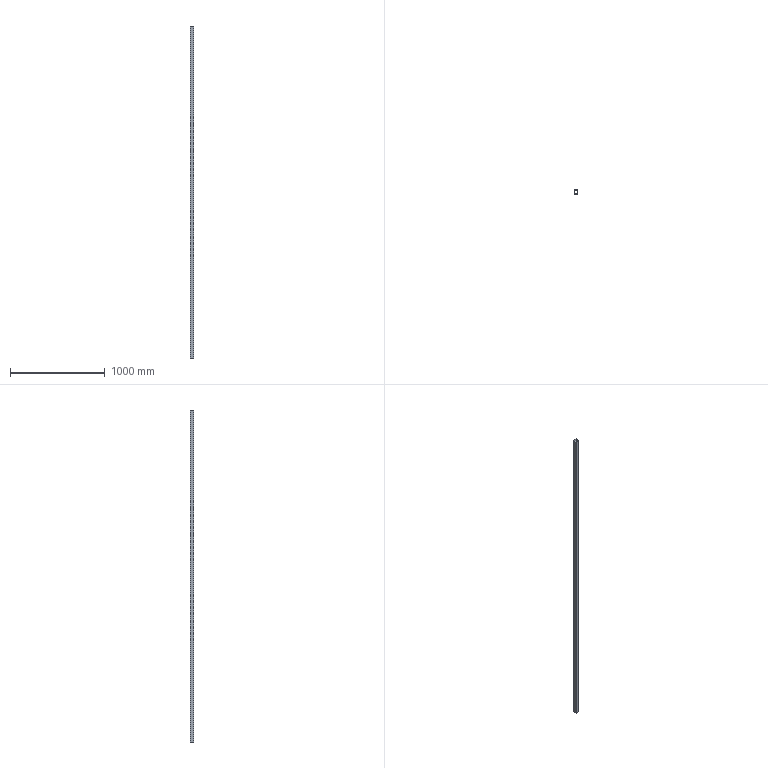Part | STEP file | BCC3 H18_1 | 1 solid | 10 faces | box 40 x 40 x 3500 mm | volume 1554000 mm3 | plane 10
STEP:
#1=CARTESIAN_POINT('',(0.,0.,0.));
#2=DIRECTION('',(0.,0.,1.));
#3=DIRECTION('',(1.,0.,0.));
#4=AXIS2_PLACEMENT_3D('',#1,#2,#3);
#5=CARTESIAN_POINT('',(-20.,20.,1750.));
#6=VERTEX_POINT('',#5);
#7=CARTESIAN_POINT('',(-20.,-20.,1750.));
#8=VERTEX_POINT('',#7);
#9=CARTESIAN_POINT('',(-20.,20.,1750.));
#10=DIRECTION('',(0.,-1.,0.));
#11=VECTOR('',#10,1.);
#12=LINE('',#9,#11);
#13=CARTESIAN_POINT('',(0.,0.,1750.));
#14=DIRECTION('',(0.,0.,1.));
#15=DIRECTION('',(1.,0.,0.));
#16=AXIS2_PLACEMENT_3D('',#13,#14,#15);
#17=PLANE('',#16);
#18=CARTESIAN_POINT('',(-20.,20.));
#19=DIRECTION('',(0.,-1.));
#20=VECTOR('',#19,1.);
#21=LINE('',#18,#20);
#22=(GEOMETRIC_REPRESENTATION_CONTEXT(2)PARAMETRIC_REPRESENTATION_CONTEXT()REPRESENTATION_CONTEXT('',''));
#23=DEFINITIONAL_REPRESENTATION('',(#21),#22);
#24=PCURVE('',#17,#23);
#25=CARTESIAN_POINT('',(-20.,20.,1750.));
#26=DIRECTION('',(1.,0.,0.));
#27=DIRECTION('',(0.,1.,0.));
#28=AXIS2_PLACEMENT_3D('',#25,#26,#27);
#29=PLANE('',#28);
#30=CARTESIAN_POINT('',(0.,0.));
#31=DIRECTION('',(-1.,0.));
#32=VECTOR('',#31,1.);
#33=LINE('',#30,#32);
#34=(GEOMETRIC_REPRESENTATION_CONTEXT(2)PARAMETRIC_REPRESENTATION_CONTEXT()REPRESENTATION_CONTEXT('',''));
#35=DEFINITIONAL_REPRESENTATION('',(#33),#34);
#36=PCURVE('',#29,#35);
#37=SURFACE_CURVE('',#12,(#24,#36),.PCURVE_S1.);
#38=EDGE_CURVE('',#6,#8,#37,.T.);
#39=ORIENTED_EDGE('',*,*,#38,.T.);
#40=CARTESIAN_POINT('',(20.,-20.,1750.));
#41=VERTEX_POINT('',#40);
#42=CARTESIAN_POINT('',(-20.,-20.,1750.));
#43=DIRECTION('',(1.,0.,0.));
#44=VECTOR('',#43,1.);
#45=LINE('',#42,#44);
#46=CARTESIAN_POINT('',(-20.,-20.));
#47=DIRECTION('',(1.,0.));
#48=VECTOR('',#47,1.);
#49=LINE('',#46,#48);
#50=(GEOMETRIC_REPRESENTATION_CONTEXT(2)PARAMETRIC_REPRESENTATION_CONTEXT()REPRESENTATION_CONTEXT('',''));
#51=DEFINITIONAL_REPRESENTATION('',(#49),#50);
#52=PCURVE('',#17,#51);
#53=CARTESIAN_POINT('',(-20.,-20.,1750.));
#54=DIRECTION('',(0.,1.,0.));
#55=DIRECTION('',(0.,0.,1.));
#56=AXIS2_PLACEMENT_3D('',#53,#54,#55);
#57=PLANE('',#56);
#58=CARTESIAN_POINT('',(0.,0.));
#59=DIRECTION('',(0.,1.));
#60=VECTOR('',#59,1.);
#61=LINE('',#58,#60);
#62=(GEOMETRIC_REPRESENTATION_CONTEXT(2)PARAMETRIC_REPRESENTATION_CONTEXT()REPRESENTATION_CONTEXT('',''));
#63=DEFINITIONAL_REPRESENTATION('',(#61),#62);
#64=PCURVE('',#57,#63);
#65=SURFACE_CURVE('',#45,(#52,#64),.PCURVE_S1.);
#66=EDGE_CURVE('',#8,#41,#65,.T.);
#67=ORIENTED_EDGE('',*,*,#66,.T.);
#68=CARTESIAN_POINT('',(20.,20.,1750.));
#69=VERTEX_POINT('',#68);
#70=CARTESIAN_POINT('',(20.,20.,1750.));
#71=DIRECTION('',(0.,1.,0.));
#72=VECTOR('',#71,1.);
#73=LINE('',#70,#72);
#74=CARTESIAN_POINT('',(20.,20.));
#75=DIRECTION('',(0.,1.));
#76=VECTOR('',#75,1.);
#77=LINE('',#74,#76);
#78=(GEOMETRIC_REPRESENTATION_CONTEXT(2)PARAMETRIC_REPRESENTATION_CONTEXT()REPRESENTATION_CONTEXT('',''));
#79=DEFINITIONAL_REPRESENTATION('',(#77),#78);
#80=PCURVE('',#17,#79);
#81=CARTESIAN_POINT('',(20.,20.,1750.));
#82=DIRECTION('',(-1.,0.,0.));
#83=DIRECTION('',(0.,-1.,0.));
#84=AXIS2_PLACEMENT_3D('',#81,#82,#83);
#85=PLANE('',#84);
#86=CARTESIAN_POINT('',(0.,0.));
#87=DIRECTION('',(-1.,0.));
#88=VECTOR('',#87,1.);
#89=LINE('',#86,#88);
#90=(GEOMETRIC_REPRESENTATION_CONTEXT(2)PARAMETRIC_REPRESENTATION_CONTEXT()REPRESENTATION_CONTEXT('',''));
#91=DEFINITIONAL_REPRESENTATION('',(#89),#90);
#92=PCURVE('',#85,#91);
#93=SURFACE_CURVE('',#73,(#80,#92),.PCURVE_S1.);
#94=EDGE_CURVE('',#41,#69,#93,.T.);
#95=ORIENTED_EDGE('',*,*,#94,.T.);
#96=CARTESIAN_POINT('',(-20.,20.,1750.));
#97=DIRECTION('',(-1.,0.,0.));
#98=VECTOR('',#97,1.);
#99=LINE('',#96,#98);
#100=CARTESIAN_POINT('',(-20.,20.));
#101=DIRECTION('',(-1.,0.));
#102=VECTOR('',#101,1.);
#103=LINE('',#100,#102);
#104=(GEOMETRIC_REPRESENTATION_CONTEXT(2)PARAMETRIC_REPRESENTATION_CONTEXT()REPRESENTATION_CONTEXT('',''));
#105=DEFINITIONAL_REPRESENTATION('',(#103),#104);
#106=PCURVE('',#17,#105);
#107=CARTESIAN_POINT('',(-20.,20.,1750.));
#108=DIRECTION('',(0.,-1.,0.));
#109=DIRECTION('',(0.,0.,-1.));
#110=AXIS2_PLACEMENT_3D('',#107,#108,#109);
#111=PLANE('',#110);
#112=CARTESIAN_POINT('',(0.,0.));
#113=DIRECTION('',(0.,-1.));
#114=VECTOR('',#113,1.);
#115=LINE('',#112,#114);
#116=(GEOMETRIC_REPRESENTATION_CONTEXT(2)PARAMETRIC_REPRESENTATION_CONTEXT()REPRESENTATION_CONTEXT('',''));
#117=DEFINITIONAL_REPRESENTATION('',(#115),#116);
#118=PCURVE('',#111,#117);
#119=SURFACE_CURVE('',#99,(#106,#118),.PCURVE_S1.);
#120=EDGE_CURVE('',#69,#6,#119,.T.);
#121=ORIENTED_EDGE('',*,*,#120,.T.);
#122=EDGE_LOOP('',(#39,#67,#95,#121));
#123=FACE_BOUND('',#122,.T.);
#124=CARTESIAN_POINT('',(-17.,-17.,1750.));
#125=VERTEX_POINT('',#124);
#126=CARTESIAN_POINT('',(17.,-17.,1750.));
#127=VERTEX_POINT('',#126);
#128=CARTESIAN_POINT('',(-17.,-17.,1750.));
#129=DIRECTION('',(1.,0.,0.));
#130=VECTOR('',#129,1.);
#131=LINE('',#128,#130);
#132=CARTESIAN_POINT('',(-17.,-17.));
#133=DIRECTION('',(1.,0.));
#134=VECTOR('',#133,1.);
#135=LINE('',#132,#134);
#136=(GEOMETRIC_REPRESENTATION_CONTEXT(2)PARAMETRIC_REPRESENTATION_CONTEXT()REPRESENTATION_CONTEXT('',''));
#137=DEFINITIONAL_REPRESENTATION('',(#135),#136);
#138=PCURVE('',#17,#137);
#139=CARTESIAN_POINT('',(-17.,-17.,1750.));
#140=DIRECTION('',(0.,1.,0.));
#141=DIRECTION('',(-1.,0.,0.));
#142=AXIS2_PLACEMENT_3D('',#139,#140,#141);
#143=PLANE('',#142);
#144=CARTESIAN_POINT('',(0.,0.));
#145=DIRECTION('',(-1.,0.));
#146=VECTOR('',#145,1.);
#147=LINE('',#144,#146);
#148=(GEOMETRIC_REPRESENTATION_CONTEXT(2)PARAMETRIC_REPRESENTATION_CONTEXT()REPRESENTATION_CONTEXT('',''));
#149=DEFINITIONAL_REPRESENTATION('',(#147),#148);
#150=PCURVE('',#143,#149);
#151=SURFACE_CURVE('',#131,(#138,#150),.PCURVE_S1.);
#152=EDGE_CURVE('',#125,#127,#151,.T.);
#153=ORIENTED_EDGE('',*,*,#152,.F.);
#154=CARTESIAN_POINT('',(-17.,17.,1750.));
#155=VERTEX_POINT('',#154);
#156=CARTESIAN_POINT('',(-17.,17.,1750.));
#157=DIRECTION('',(0.,-1.,0.));
#158=VECTOR('',#157,1.);
#159=LINE('',#156,#158);
#160=CARTESIAN_POINT('',(-17.,17.));
#161=DIRECTION('',(0.,-1.));
#162=VECTOR('',#161,1.);
#163=LINE('',#160,#162);
#164=(GEOMETRIC_REPRESENTATION_CONTEXT(2)PARAMETRIC_REPRESENTATION_CONTEXT()REPRESENTATION_CONTEXT('',''));
#165=DEFINITIONAL_REPRESENTATION('',(#163),#164);
#166=PCURVE('',#17,#165);
#167=CARTESIAN_POINT('',(-17.,17.,1750.));
#168=DIRECTION('',(1.,0.,0.));
#169=DIRECTION('',(0.,1.,0.));
#170=AXIS2_PLACEMENT_3D('',#167,#168,#169);
#171=PLANE('',#170);
#172=CARTESIAN_POINT('',(0.,0.));
#173=DIRECTION('',(-1.,0.));
#174=VECTOR('',#173,1.);
#175=LINE('',#172,#174);
#176=(GEOMETRIC_REPRESENTATION_CONTEXT(2)PARAMETRIC_REPRESENTATION_CONTEXT()REPRESENTATION_CONTEXT('',''));
#177=DEFINITIONAL_REPRESENTATION('',(#175),#176);
#178=PCURVE('',#171,#177);
#179=SURFACE_CURVE('',#159,(#166,#178),.PCURVE_S1.);
#180=EDGE_CURVE('',#155,#125,#179,.T.);
#181=ORIENTED_EDGE('',*,*,#180,.F.);
#182=CARTESIAN_POINT('',(17.,17.,1750.));
#183=VERTEX_POINT('',#182);
#184=CARTESIAN_POINT('',(-17.,17.,1750.));
#185=DIRECTION('',(-1.,0.,0.));
#186=VECTOR('',#185,1.);
#187=LINE('',#184,#186);
#188=CARTESIAN_POINT('',(-17.,17.));
#189=DIRECTION('',(-1.,0.));
#190=VECTOR('',#189,1.);
#191=LINE('',#188,#190);
#192=(GEOMETRIC_REPRESENTATION_CONTEXT(2)PARAMETRIC_REPRESENTATION_CONTEXT()REPRESENTATION_CONTEXT('',''));
#193=DEFINITIONAL_REPRESENTATION('',(#191),#192);
#194=PCURVE('',#17,#193);
#195=CARTESIAN_POINT('',(-17.,17.,1750.));
#196=DIRECTION('',(0.,-1.,0.));
#197=DIRECTION('',(0.,0.,-1.));
#198=AXIS2_PLACEMENT_3D('',#195,#196,#197);
#199=PLANE('',#198);
#200=CARTESIAN_POINT('',(0.,0.));
#201=DIRECTION('',(0.,-1.));
#202=VECTOR('',#201,1.);
#203=LINE('',#200,#202);
#204=(GEOMETRIC_REPRESENTATION_CONTEXT(2)PARAMETRIC_REPRESENTATION_CONTEXT()REPRESENTATION_CONTEXT('',''));
#205=DEFINITIONAL_REPRESENTATION('',(#203),#204);
#206=PCURVE('',#199,#205);
#207=SURFACE_CURVE('',#187,(#194,#206),.PCURVE_S1.);
#208=EDGE_CURVE('',#183,#155,#207,.T.);
#209=ORIENTED_EDGE('',*,*,#208,.F.);
#210=CARTESIAN_POINT('',(17.,17.,1750.));
#211=DIRECTION('',(0.,1.,0.));
#212=VECTOR('',#211,1.);
#213=LINE('',#210,#212);
#214=CARTESIAN_POINT('',(17.,17.));
#215=DIRECTION('',(0.,1.));
#216=VECTOR('',#215,1.);
#217=LINE('',#214,#216);
#218=(GEOMETRIC_REPRESENTATION_CONTEXT(2)PARAMETRIC_REPRESENTATION_CONTEXT()REPRESENTATION_CONTEXT('',''));
#219=DEFINITIONAL_REPRESENTATION('',(#217),#218);
#220=PCURVE('',#17,#219);
#221=CARTESIAN_POINT('',(17.,17.,1750.));
#222=DIRECTION('',(-1.,0.,0.));
#223=DIRECTION('',(0.,-1.,0.));
#224=AXIS2_PLACEMENT_3D('',#221,#222,#223);
#225=PLANE('',#224);
#226=CARTESIAN_POINT('',(0.,0.));
#227=DIRECTION('',(-1.,0.));
#228=VECTOR('',#227,1.);
#229=LINE('',#226,#228);
#230=(GEOMETRIC_REPRESENTATION_CONTEXT(2)PARAMETRIC_REPRESENTATION_CONTEXT()REPRESENTATION_CONTEXT('',''));
#231=DEFINITIONAL_REPRESENTATION('',(#229),#230);
#232=PCURVE('',#225,#231);
#233=SURFACE_CURVE('',#213,(#220,#232),.PCURVE_S1.);
#234=EDGE_CURVE('',#127,#183,#233,.T.);
#235=ORIENTED_EDGE('',*,*,#234,.F.);
#236=EDGE_LOOP('',(#153,#181,#209,#235));
#237=FACE_BOUND('',#236,.T.);
#238=ADVANCED_FACE('',(#123,#237),#17,.T.);
#239=CARTESIAN_POINT('',(-20.,20.,-1750.));
#240=VERTEX_POINT('',#239);
#241=CARTESIAN_POINT('',(-20.,-20.,-1750.));
#242=VERTEX_POINT('',#241);
#243=CARTESIAN_POINT('',(-20.,20.,-1750.));
#244=DIRECTION('',(0.,-1.,0.));
#245=VECTOR('',#244,1.);
#246=LINE('',#243,#245);
#247=CARTESIAN_POINT('',(0.,0.,-1750.));
#248=DIRECTION('',(0.,0.,1.));
#249=DIRECTION('',(1.,0.,0.));
#250=AXIS2_PLACEMENT_3D('',#247,#248,#249);
#251=PLANE('',#250);
#252=CARTESIAN_POINT('',(-20.,20.));
#253=DIRECTION('',(0.,-1.));
#254=VECTOR('',#253,1.);
#255=LINE('',#252,#254);
#256=(GEOMETRIC_REPRESENTATION_CONTEXT(2)PARAMETRIC_REPRESENTATION_CONTEXT()REPRESENTATION_CONTEXT('',''));
#257=DEFINITIONAL_REPRESENTATION('',(#255),#256);
#258=PCURVE('',#251,#257);
#259=CARTESIAN_POINT('',(0.,-3500.));
#260=DIRECTION('',(-1.,0.));
#261=VECTOR('',#260,1.);
#262=LINE('',#259,#261);
#263=(GEOMETRIC_REPRESENTATION_CONTEXT(2)PARAMETRIC_REPRESENTATION_CONTEXT()REPRESENTATION_CONTEXT('',''));
#264=DEFINITIONAL_REPRESENTATION('',(#262),#263);
#265=PCURVE('',#29,#264);
#266=SURFACE_CURVE('',#246,(#258,#265),.PCURVE_S1.);
#267=EDGE_CURVE('',#240,#242,#266,.T.);
#268=ORIENTED_EDGE('',*,*,#267,.F.);
#269=CARTESIAN_POINT('',(20.,20.,-1750.));
#270=VERTEX_POINT('',#269);
#271=CARTESIAN_POINT('',(-20.,20.,-1750.));
#272=DIRECTION('',(-1.,0.,0.));
#273=VECTOR('',#272,1.);
#274=LINE('',#271,#273);
#275=CARTESIAN_POINT('',(-20.,20.));
#276=DIRECTION('',(-1.,0.));
#277=VECTOR('',#276,1.);
#278=LINE('',#275,#277);
#279=(GEOMETRIC_REPRESENTATION_CONTEXT(2)PARAMETRIC_REPRESENTATION_CONTEXT()REPRESENTATION_CONTEXT('',''));
#280=DEFINITIONAL_REPRESENTATION('',(#278),#279);
#281=PCURVE('',#251,#280);
#282=CARTESIAN_POINT('',(3500.,0.));
#283=DIRECTION('',(0.,-1.));
#284=VECTOR('',#283,1.);
#285=LINE('',#282,#284);
#286=(GEOMETRIC_REPRESENTATION_CONTEXT(2)PARAMETRIC_REPRESENTATION_CONTEXT()REPRESENTATION_CONTEXT('',''));
#287=DEFINITIONAL_REPRESENTATION('',(#285),#286);
#288=PCURVE('',#111,#287);
#289=SURFACE_CURVE('',#274,(#281,#288),.PCURVE_S1.);
#290=EDGE_CURVE('',#270,#240,#289,.T.);
#291=ORIENTED_EDGE('',*,*,#290,.F.);
#292=CARTESIAN_POINT('',(20.,-20.,-1750.));
#293=VERTEX_POINT('',#292);
#294=CARTESIAN_POINT('',(20.,20.,-1750.));
#295=DIRECTION('',(0.,1.,0.));
#296=VECTOR('',#295,1.);
#297=LINE('',#294,#296);
#298=CARTESIAN_POINT('',(20.,20.));
#299=DIRECTION('',(0.,1.));
#300=VECTOR('',#299,1.);
#301=LINE('',#298,#300);
#302=(GEOMETRIC_REPRESENTATION_CONTEXT(2)PARAMETRIC_REPRESENTATION_CONTEXT()REPRESENTATION_CONTEXT('',''));
#303=DEFINITIONAL_REPRESENTATION('',(#301),#302);
#304=PCURVE('',#251,#303);
#305=CARTESIAN_POINT('',(0.,-3500.));
#306=DIRECTION('',(-1.,0.));
#307=VECTOR('',#306,1.);
#308=LINE('',#305,#307);
#309=(GEOMETRIC_REPRESENTATION_CONTEXT(2)PARAMETRIC_REPRESENTATION_CONTEXT()REPRESENTATION_CONTEXT('',''));
#310=DEFINITIONAL_REPRESENTATION('',(#308),#309);
#311=PCURVE('',#85,#310);
#312=SURFACE_CURVE('',#297,(#304,#311),.PCURVE_S1.);
#313=EDGE_CURVE('',#293,#270,#312,.T.);
#314=ORIENTED_EDGE('',*,*,#313,.F.);
#315=CARTESIAN_POINT('',(-20.,-20.,-1750.));
#316=DIRECTION('',(1.,0.,0.));
#317=VECTOR('',#316,1.);
#318=LINE('',#315,#317);
#319=CARTESIAN_POINT('',(-20.,-20.));
#320=DIRECTION('',(1.,0.));
#321=VECTOR('',#320,1.);
#322=LINE('',#319,#321);
#323=(GEOMETRIC_REPRESENTATION_CONTEXT(2)PARAMETRIC_REPRESENTATION_CONTEXT()REPRESENTATION_CONTEXT('',''));
#324=DEFINITIONAL_REPRESENTATION('',(#322),#323);
#325=PCURVE('',#251,#324);
#326=CARTESIAN_POINT('',(-3500.,0.));
#327=DIRECTION('',(0.,1.));
#328=VECTOR('',#327,1.);
#329=LINE('',#326,#328);
#330=(GEOMETRIC_REPRESENTATION_CONTEXT(2)PARAMETRIC_REPRESENTATION_CONTEXT()REPRESENTATION_CONTEXT('',''));
#331=DEFINITIONAL_REPRESENTATION('',(#329),#330);
#332=PCURVE('',#57,#331);
#333=SURFACE_CURVE('',#318,(#325,#332),.PCURVE_S1.);
#334=EDGE_CURVE('',#242,#293,#333,.T.);
#335=ORIENTED_EDGE('',*,*,#334,.F.);
#336=EDGE_LOOP('',(#268,#291,#314,#335));
#337=FACE_BOUND('',#336,.T.);
#338=CARTESIAN_POINT('',(-17.,17.,-1750.));
#339=VERTEX_POINT('',#338);
#340=CARTESIAN_POINT('',(-17.,-17.,-1750.));
#341=VERTEX_POINT('',#340);
#342=CARTESIAN_POINT('',(-17.,17.,-1750.));
#343=DIRECTION('',(0.,-1.,0.));
#344=VECTOR('',#343,1.);
#345=LINE('',#342,#344);
#346=CARTESIAN_POINT('',(-17.,17.));
#347=DIRECTION('',(0.,-1.));
#348=VECTOR('',#347,1.);
#349=LINE('',#346,#348);
#350=(GEOMETRIC_REPRESENTATION_CONTEXT(2)PARAMETRIC_REPRESENTATION_CONTEXT()REPRESENTATION_CONTEXT('',''));
#351=DEFINITIONAL_REPRESENTATION('',(#349),#350);
#352=PCURVE('',#251,#351);
#353=CARTESIAN_POINT('',(0.,-3500.));
#354=DIRECTION('',(-1.,0.));
#355=VECTOR('',#354,1.);
#356=LINE('',#353,#355);
#357=(GEOMETRIC_REPRESENTATION_CONTEXT(2)PARAMETRIC_REPRESENTATION_CONTEXT()REPRESENTATION_CONTEXT('',''));
#358=DEFINITIONAL_REPRESENTATION('',(#356),#357);
#359=PCURVE('',#171,#358);
#360=SURFACE_CURVE('',#345,(#352,#359),.PCURVE_S1.);
#361=EDGE_CURVE('',#339,#341,#360,.T.);
#362=ORIENTED_EDGE('',*,*,#361,.T.);
#363=CARTESIAN_POINT('',(17.,-17.,-1750.));
#364=VERTEX_POINT('',#363);
#365=CARTESIAN_POINT('',(-17.,-17.,-1750.));
#366=DIRECTION('',(1.,0.,0.));
#367=VECTOR('',#366,1.);
#368=LINE('',#365,#367);
#369=CARTESIAN_POINT('',(-17.,-17.));
#370=DIRECTION('',(1.,0.));
#371=VECTOR('',#370,1.);
#372=LINE('',#369,#371);
#373=(GEOMETRIC_REPRESENTATION_CONTEXT(2)PARAMETRIC_REPRESENTATION_CONTEXT()REPRESENTATION_CONTEXT('',''));
#374=DEFINITIONAL_REPRESENTATION('',(#372),#373);
#375=PCURVE('',#251,#374);
#376=CARTESIAN_POINT('',(0.,-3500.));
#377=DIRECTION('',(-1.,0.));
#378=VECTOR('',#377,1.);
#379=LINE('',#376,#378);
#380=(GEOMETRIC_REPRESENTATION_CONTEXT(2)PARAMETRIC_REPRESENTATION_CONTEXT()REPRESENTATION_CONTEXT('',''));
#381=DEFINITIONAL_REPRESENTATION('',(#379),#380);
#382=PCURVE('',#143,#381);
#383=SURFACE_CURVE('',#368,(#375,#382),.PCURVE_S1.);
#384=EDGE_CURVE('',#341,#364,#383,.T.);
#385=ORIENTED_EDGE('',*,*,#384,.T.);
#386=CARTESIAN_POINT('',(17.,17.,-1750.));
#387=VERTEX_POINT('',#386);
#388=CARTESIAN_POINT('',(17.,17.,-1750.));
#389=DIRECTION('',(0.,1.,0.));
#390=VECTOR('',#389,1.);
#391=LINE('',#388,#390);
#392=CARTESIAN_POINT('',(17.,17.));
#393=DIRECTION('',(0.,1.));
#394=VECTOR('',#393,1.);
#395=LINE('',#392,#394);
#396=(GEOMETRIC_REPRESENTATION_CONTEXT(2)PARAMETRIC_REPRESENTATION_CONTEXT()REPRESENTATION_CONTEXT('',''));
#397=DEFINITIONAL_REPRESENTATION('',(#395),#396);
#398=PCURVE('',#251,#397);
#399=CARTESIAN_POINT('',(0.,-3500.));
#400=DIRECTION('',(-1.,0.));
#401=VECTOR('',#400,1.);
#402=LINE('',#399,#401);
#403=(GEOMETRIC_REPRESENTATION_CONTEXT(2)PARAMETRIC_REPRESENTATION_CONTEXT()REPRESENTATION_CONTEXT('',''));
#404=DEFINITIONAL_REPRESENTATION('',(#402),#403);
#405=PCURVE('',#225,#404);
#406=SURFACE_CURVE('',#391,(#398,#405),.PCURVE_S1.);
#407=EDGE_CURVE('',#364,#387,#406,.T.);
#408=ORIENTED_EDGE('',*,*,#407,.T.);
#409=CARTESIAN_POINT('',(-17.,17.,-1750.));
#410=DIRECTION('',(-1.,0.,0.));
#411=VECTOR('',#410,1.);
#412=LINE('',#409,#411);
#413=CARTESIAN_POINT('',(-17.,17.));
#414=DIRECTION('',(-1.,0.));
#415=VECTOR('',#414,1.);
#416=LINE('',#413,#415);
#417=(GEOMETRIC_REPRESENTATION_CONTEXT(2)PARAMETRIC_REPRESENTATION_CONTEXT()REPRESENTATION_CONTEXT('',''));
#418=DEFINITIONAL_REPRESENTATION('',(#416),#417);
#419=PCURVE('',#251,#418);
#420=CARTESIAN_POINT('',(3500.,0.));
#421=DIRECTION('',(0.,-1.));
#422=VECTOR('',#421,1.);
#423=LINE('',#420,#422);
#424=(GEOMETRIC_REPRESENTATION_CONTEXT(2)PARAMETRIC_REPRESENTATION_CONTEXT()REPRESENTATION_CONTEXT('',''));
#425=DEFINITIONAL_REPRESENTATION('',(#423),#424);
#426=PCURVE('',#199,#425);
#427=SURFACE_CURVE('',#412,(#419,#426),.PCURVE_S1.);
#428=EDGE_CURVE('',#387,#339,#427,.T.);
#429=ORIENTED_EDGE('',*,*,#428,.T.);
#430=EDGE_LOOP('',(#362,#385,#408,#429));
#431=FACE_BOUND('',#430,.T.);
#432=ADVANCED_FACE('',(#337,#431),#251,.F.);
#433=ORIENTED_EDGE('',*,*,#267,.T.);
#434=CARTESIAN_POINT('',(-20.,-20.,1750.));
#435=DIRECTION('',(0.,0.,-1.));
#436=VECTOR('',#435,1.);
#437=LINE('',#434,#436);
#438=CARTESIAN_POINT('',(-40.,0.));
#439=DIRECTION('',(0.,-1.));
#440=VECTOR('',#439,1.);
#441=LINE('',#438,#440);
#442=(GEOMETRIC_REPRESENTATION_CONTEXT(2)PARAMETRIC_REPRESENTATION_CONTEXT()REPRESENTATION_CONTEXT('',''));
#443=DEFINITIONAL_REPRESENTATION('',(#441),#442);
#444=PCURVE('',#29,#443);
#445=CARTESIAN_POINT('',(0.,0.));
#446=DIRECTION('',(-1.,0.));
#447=VECTOR('',#446,1.);
#448=LINE('',#445,#447);
#449=(GEOMETRIC_REPRESENTATION_CONTEXT(2)PARAMETRIC_REPRESENTATION_CONTEXT()REPRESENTATION_CONTEXT('',''));
#450=DEFINITIONAL_REPRESENTATION('',(#448),#449);
#451=PCURVE('',#57,#450);
#452=SURFACE_CURVE('',#437,(#444,#451),.PCURVE_S1.);
#453=EDGE_CURVE('',#8,#242,#452,.T.);
#454=ORIENTED_EDGE('',*,*,#453,.F.);
#455=ORIENTED_EDGE('',*,*,#38,.F.);
#456=CARTESIAN_POINT('',(-20.,20.,1750.));
#457=DIRECTION('',(0.,0.,-1.));
#458=VECTOR('',#457,1.);
#459=LINE('',#456,#458);
#460=CARTESIAN_POINT('',(0.,0.));
#461=DIRECTION('',(0.,-1.));
#462=VECTOR('',#461,1.);
#463=LINE('',#460,#462);
#464=(GEOMETRIC_REPRESENTATION_CONTEXT(2)PARAMETRIC_REPRESENTATION_CONTEXT()REPRESENTATION_CONTEXT('',''));
#465=DEFINITIONAL_REPRESENTATION('',(#463),#464);
#466=PCURVE('',#29,#465);
#467=CARTESIAN_POINT('',(0.,0.));
#468=DIRECTION('',(1.,0.));
#469=VECTOR('',#468,1.);
#470=LINE('',#467,#469);
#471=(GEOMETRIC_REPRESENTATION_CONTEXT(2)PARAMETRIC_REPRESENTATION_CONTEXT()REPRESENTATION_CONTEXT('',''));
#472=DEFINITIONAL_REPRESENTATION('',(#470),#471);
#473=PCURVE('',#111,#472);
#474=SURFACE_CURVE('',#459,(#466,#473),.PCURVE_S1.);
#475=EDGE_CURVE('',#6,#240,#474,.T.);
#476=ORIENTED_EDGE('',*,*,#475,.T.);
#477=EDGE_LOOP('',(#433,#454,#455,#476));
#478=FACE_BOUND('',#477,.T.);
#479=ADVANCED_FACE('',(#478),#29,.F.);
#480=ORIENTED_EDGE('',*,*,#334,.T.);
#481=CARTESIAN_POINT('',(20.,-20.,1750.));
#482=DIRECTION('',(0.,0.,-1.));
#483=VECTOR('',#482,1.);
#484=LINE('',#481,#483);
#485=CARTESIAN_POINT('',(0.,40.));
#486=DIRECTION('',(-1.,0.));
#487=VECTOR('',#486,1.);
#488=LINE('',#485,#487);
#489=(GEOMETRIC_REPRESENTATION_CONTEXT(2)PARAMETRIC_REPRESENTATION_CONTEXT()REPRESENTATION_CONTEXT('',''));
#490=DEFINITIONAL_REPRESENTATION('',(#488),#489);
#491=PCURVE('',#57,#490);
#492=CARTESIAN_POINT('',(40.,0.));
#493=DIRECTION('',(0.,-1.));
#494=VECTOR('',#493,1.);
#495=LINE('',#492,#494);
#496=(GEOMETRIC_REPRESENTATION_CONTEXT(2)PARAMETRIC_REPRESENTATION_CONTEXT()REPRESENTATION_CONTEXT('',''));
#497=DEFINITIONAL_REPRESENTATION('',(#495),#496);
#498=PCURVE('',#85,#497);
#499=SURFACE_CURVE('',#484,(#491,#498),.PCURVE_S1.);
#500=EDGE_CURVE('',#41,#293,#499,.T.);
#501=ORIENTED_EDGE('',*,*,#500,.F.);
#502=ORIENTED_EDGE('',*,*,#66,.F.);
#503=ORIENTED_EDGE('',*,*,#453,.T.);
#504=EDGE_LOOP('',(#480,#501,#502,#503));
#505=FACE_BOUND('',#504,.T.);
#506=ADVANCED_FACE('',(#505),#57,.F.);
#507=ORIENTED_EDGE('',*,*,#313,.T.);
#508=CARTESIAN_POINT('',(20.,20.,1750.));
#509=DIRECTION('',(0.,0.,-1.));
#510=VECTOR('',#509,1.);
#511=LINE('',#508,#510);
#512=CARTESIAN_POINT('',(0.,0.));
#513=DIRECTION('',(0.,-1.));
#514=VECTOR('',#513,1.);
#515=LINE('',#512,#514);
#516=(GEOMETRIC_REPRESENTATION_CONTEXT(2)PARAMETRIC_REPRESENTATION_CONTEXT()REPRESENTATION_CONTEXT('',''));
#517=DEFINITIONAL_REPRESENTATION('',(#515),#516);
#518=PCURVE('',#85,#517);
#519=CARTESIAN_POINT('',(0.,40.));
#520=DIRECTION('',(1.,0.));
#521=VECTOR('',#520,1.);
#522=LINE('',#519,#521);
#523=(GEOMETRIC_REPRESENTATION_CONTEXT(2)PARAMETRIC_REPRESENTATION_CONTEXT()REPRESENTATION_CONTEXT('',''));
#524=DEFINITIONAL_REPRESENTATION('',(#522),#523);
#525=PCURVE('',#111,#524);
#526=SURFACE_CURVE('',#511,(#518,#525),.PCURVE_S1.);
#527=EDGE_CURVE('',#69,#270,#526,.T.);
#528=ORIENTED_EDGE('',*,*,#527,.F.);
#529=ORIENTED_EDGE('',*,*,#94,.F.);
#530=ORIENTED_EDGE('',*,*,#500,.T.);
#531=EDGE_LOOP('',(#507,#528,#529,#530));
#532=FACE_BOUND('',#531,.T.);
#533=ADVANCED_FACE('',(#532),#85,.F.);
#534=ORIENTED_EDGE('',*,*,#290,.T.);
#535=ORIENTED_EDGE('',*,*,#475,.F.);
#536=ORIENTED_EDGE('',*,*,#120,.F.);
#537=ORIENTED_EDGE('',*,*,#527,.T.);
#538=EDGE_LOOP('',(#534,#535,#536,#537));
#539=FACE_BOUND('',#538,.T.);
#540=ADVANCED_FACE('',(#539),#111,.F.);
#541=ORIENTED_EDGE('',*,*,#361,.F.);
#542=CARTESIAN_POINT('',(-17.,17.,1750.));
#543=DIRECTION('',(0.,0.,-1.));
#544=VECTOR('',#543,1.);
#545=LINE('',#542,#544);
#546=CARTESIAN_POINT('',(0.,0.));
#547=DIRECTION('',(0.,-1.));
#548=VECTOR('',#547,1.);
#549=LINE('',#546,#548);
#550=(GEOMETRIC_REPRESENTATION_CONTEXT(2)PARAMETRIC_REPRESENTATION_CONTEXT()REPRESENTATION_CONTEXT('',''));
#551=DEFINITIONAL_REPRESENTATION('',(#549),#550);
#552=PCURVE('',#171,#551);
#553=CARTESIAN_POINT('',(0.,0.));
#554=DIRECTION('',(1.,0.));
#555=VECTOR('',#554,1.);
#556=LINE('',#553,#555);
#557=(GEOMETRIC_REPRESENTATION_CONTEXT(2)PARAMETRIC_REPRESENTATION_CONTEXT()REPRESENTATION_CONTEXT('',''));
#558=DEFINITIONAL_REPRESENTATION('',(#556),#557);
#559=PCURVE('',#199,#558);
#560=SURFACE_CURVE('',#545,(#552,#559),.PCURVE_S1.);
#561=EDGE_CURVE('',#155,#339,#560,.T.);
#562=ORIENTED_EDGE('',*,*,#561,.F.);
#563=ORIENTED_EDGE('',*,*,#180,.T.);
#564=CARTESIAN_POINT('',(-17.,-17.,1750.));
#565=DIRECTION('',(0.,0.,-1.));
#566=VECTOR('',#565,1.);
#567=LINE('',#564,#566);
#568=CARTESIAN_POINT('',(-34.,0.));
#569=DIRECTION('',(0.,-1.));
#570=VECTOR('',#569,1.);
#571=LINE('',#568,#570);
#572=(GEOMETRIC_REPRESENTATION_CONTEXT(2)PARAMETRIC_REPRESENTATION_CONTEXT()REPRESENTATION_CONTEXT('',''));
#573=DEFINITIONAL_REPRESENTATION('',(#571),#572);
#574=PCURVE('',#171,#573);
#575=CARTESIAN_POINT('',(0.,0.));
#576=DIRECTION('',(0.,-1.));
#577=VECTOR('',#576,1.);
#578=LINE('',#575,#577);
#579=(GEOMETRIC_REPRESENTATION_CONTEXT(2)PARAMETRIC_REPRESENTATION_CONTEXT()REPRESENTATION_CONTEXT('',''));
#580=DEFINITIONAL_REPRESENTATION('',(#578),#579);
#581=PCURVE('',#143,#580);
#582=SURFACE_CURVE('',#567,(#574,#581),.PCURVE_S1.);
#583=EDGE_CURVE('',#125,#341,#582,.T.);
#584=ORIENTED_EDGE('',*,*,#583,.T.);
#585=EDGE_LOOP('',(#541,#562,#563,#584));
#586=FACE_BOUND('',#585,.T.);
#587=ADVANCED_FACE('',(#586),#171,.T.);
#588=ORIENTED_EDGE('',*,*,#384,.F.);
#589=ORIENTED_EDGE('',*,*,#583,.F.);
#590=ORIENTED_EDGE('',*,*,#152,.T.);
#591=CARTESIAN_POINT('',(17.,-17.,1750.));
#592=DIRECTION('',(0.,0.,-1.));
#593=VECTOR('',#592,1.);
#594=LINE('',#591,#593);
#595=CARTESIAN_POINT('',(-34.,0.));
#596=DIRECTION('',(0.,-1.));
#597=VECTOR('',#596,1.);
#598=LINE('',#595,#597);
#599=(GEOMETRIC_REPRESENTATION_CONTEXT(2)PARAMETRIC_REPRESENTATION_CONTEXT()REPRESENTATION_CONTEXT('',''));
#600=DEFINITIONAL_REPRESENTATION('',(#598),#599);
#601=PCURVE('',#143,#600);
#602=CARTESIAN_POINT('',(34.,0.));
#603=DIRECTION('',(0.,-1.));
#604=VECTOR('',#603,1.);
#605=LINE('',#602,#604);
#606=(GEOMETRIC_REPRESENTATION_CONTEXT(2)PARAMETRIC_REPRESENTATION_CONTEXT()REPRESENTATION_CONTEXT('',''));
#607=DEFINITIONAL_REPRESENTATION('',(#605),#606);
#608=PCURVE('',#225,#607);
#609=SURFACE_CURVE('',#594,(#601,#608),.PCURVE_S1.);
#610=EDGE_CURVE('',#127,#364,#609,.T.);
#611=ORIENTED_EDGE('',*,*,#610,.T.);
#612=EDGE_LOOP('',(#588,#589,#590,#611));
#613=FACE_BOUND('',#612,.T.);
#614=ADVANCED_FACE('',(#613),#143,.T.);
#615=ORIENTED_EDGE('',*,*,#407,.F.);
#616=ORIENTED_EDGE('',*,*,#610,.F.);
#617=ORIENTED_EDGE('',*,*,#234,.T.);
#618=CARTESIAN_POINT('',(17.,17.,1750.));
#619=DIRECTION('',(0.,0.,-1.));
#620=VECTOR('',#619,1.);
#621=LINE('',#618,#620);
#622=CARTESIAN_POINT('',(0.,0.));
#623=DIRECTION('',(0.,-1.));
#624=VECTOR('',#623,1.);
#625=LINE('',#622,#624);
#626=(GEOMETRIC_REPRESENTATION_CONTEXT(2)PARAMETRIC_REPRESENTATION_CONTEXT()REPRESENTATION_CONTEXT('',''));
#627=DEFINITIONAL_REPRESENTATION('',(#625),#626);
#628=PCURVE('',#225,#627);
#629=CARTESIAN_POINT('',(0.,34.));
#630=DIRECTION('',(1.,0.));
#631=VECTOR('',#630,1.);
#632=LINE('',#629,#631);
#633=(GEOMETRIC_REPRESENTATION_CONTEXT(2)PARAMETRIC_REPRESENTATION_CONTEXT()REPRESENTATION_CONTEXT('',''));
#634=DEFINITIONAL_REPRESENTATION('',(#632),#633);
#635=PCURVE('',#199,#634);
#636=SURFACE_CURVE('',#621,(#628,#635),.PCURVE_S1.);
#637=EDGE_CURVE('',#183,#387,#636,.T.);
#638=ORIENTED_EDGE('',*,*,#637,.T.);
#639=EDGE_LOOP('',(#615,#616,#617,#638));
#640=FACE_BOUND('',#639,.T.);
#641=ADVANCED_FACE('',(#640),#225,.T.);
#642=ORIENTED_EDGE('',*,*,#428,.F.);
#643=ORIENTED_EDGE('',*,*,#637,.F.);
#644=ORIENTED_EDGE('',*,*,#208,.T.);
#645=ORIENTED_EDGE('',*,*,#561,.T.);
#646=EDGE_LOOP('',(#642,#643,#644,#645));
#647=FACE_BOUND('',#646,.T.);
#648=ADVANCED_FACE('',(#647),#199,.T.);
#649=CLOSED_SHELL('',(#238,#432,#479,#506,#533,#540,#587,#614,#641,#648));
#650=MANIFOLD_SOLID_BREP('',#649);
#651=(LENGTH_UNIT()NAMED_UNIT(*)SI_UNIT(.MILLI.,.METRE.));
#652=UNCERTAINTY_MEASURE_WITH_UNIT(LENGTH_MEASURE(0.0000001),#651,'','');
#653=(NAMED_UNIT(*)PLANE_ANGLE_UNIT()SI_UNIT($,.RADIAN.));
#654=(NAMED_UNIT(*)SI_UNIT($,.STERADIAN.)SOLID_ANGLE_UNIT());
#655=(GEOMETRIC_REPRESENTATION_CONTEXT(3)GLOBAL_UNCERTAINTY_ASSIGNED_CONTEXT((#652))GLOBAL_UNIT_ASSIGNED_CONTEXT((#651,#653,#654))REPRESENTATION_CONTEXT('',''));
#656=ADVANCED_BREP_SHAPE_REPRESENTATION('',(#4,#650),#655);